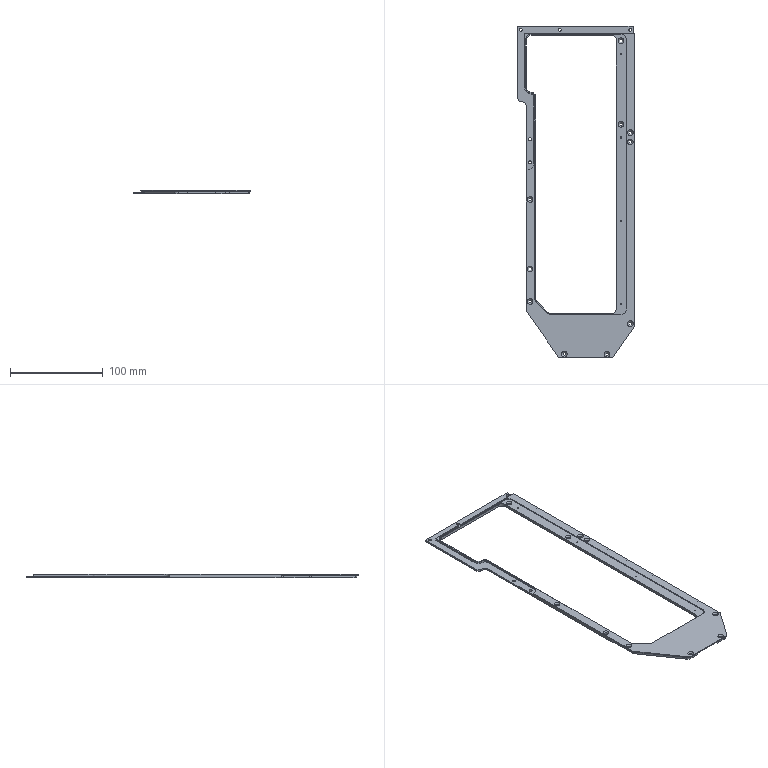NC program | NX | posted with a generic post | part box 127 x 358 x 4 mm
Whole program:
N10 G17 G21 G94 G90
(SPOT_DRILL_COPY_COPY_COPY_1 , TOOL : DRILL_D4.3-54-83)
N12 T15 M6
N14 G54
N16 G17 G0 G90 X-175. Y12.5 S3000 M3
N18 G43 Z5. H15
N20 G94 G82 G98 Z-15. F200. P200 R3.
N22 Y-33.5
N24 G80
N26 G0 X-175. Y-33.5 Z5.
N28 M5
N30 M2